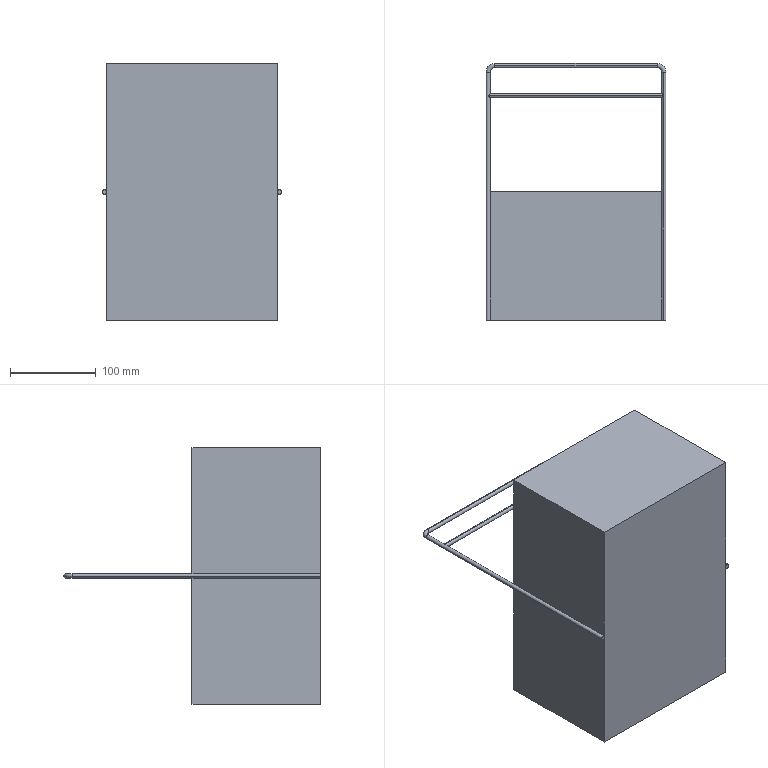Part | STEP file | 0228_Work-A | 1 solid | 21 faces | box 209.998 x 299.999 x 300 mm | volume 9019523 mm3 | cylinder 9 | plane 8 | torus 4 | commonest cylinder face diameters 5 x9